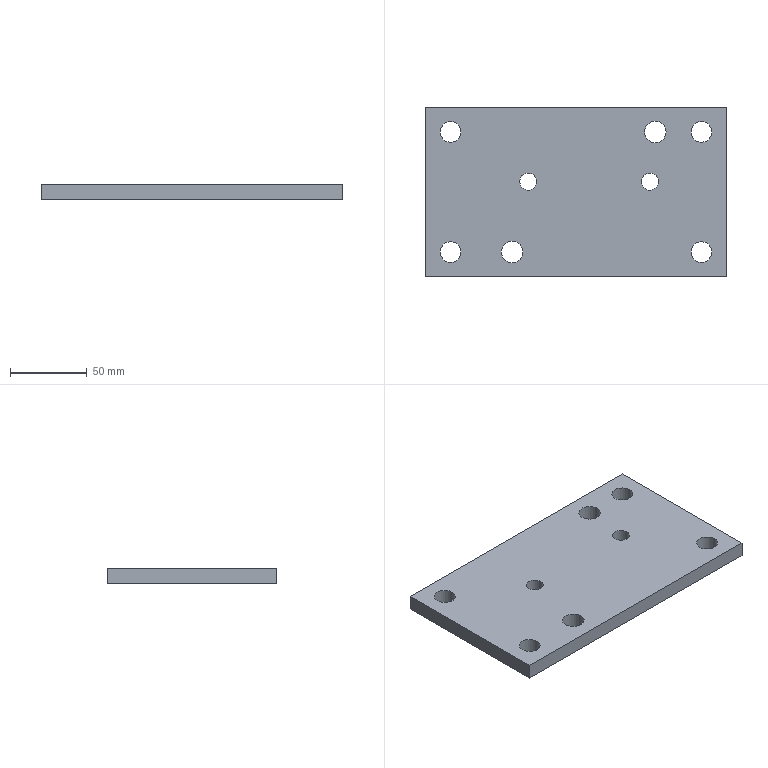Part | STEP file | lll_id2946_x_t | 1 solid | 14 faces | box 195 x 110 x 10 mm | volume 203787 mm3 | cylinder 8 | plane 6 | commonest cylinder face diameters 13.509 x4 11 x2 14 x2
STEP:
#1=CARTESIAN_POINT('',(1064.5,-23.25,102.5));
#2=VERTEX_POINT('',#1);
#3=CARTESIAN_POINT('',(1070.,-23.25,102.5));
#4=DIRECTION('',(0.,0.,-1.));
#5=DIRECTION('',(-1.,0.,0.));
#6=AXIS2_PLACEMENT_3D('',#3,#4,#5);
#7=CIRCLE('',#6,5.5);
#8=EDGE_CURVE('',#2,#2,#7,.T.);
#9=ORIENTED_EDGE('',*,*,#8,.F.);
#10=EDGE_LOOP('',(#9));
#11=FACE_BOUND('',#10,.T.);
#12=CARTESIAN_POINT('',(1064.5,-23.25,92.5));
#13=VERTEX_POINT('',#12);
#14=CARTESIAN_POINT('',(1070.,-23.25,92.5));
#15=DIRECTION('',(0.,0.,1.));
#16=DIRECTION('',(-1.,0.,0.));
#17=AXIS2_PLACEMENT_3D('',#14,#15,#16);
#18=CIRCLE('',#17,5.5);
#19=EDGE_CURVE('',#13,#13,#18,.T.);
#20=ORIENTED_EDGE('',*,*,#19,.F.);
#21=EDGE_LOOP('',(#20));
#22=FACE_BOUND('',#21,.T.);
#23=CARTESIAN_POINT('',(1070.,-23.25,217.5));
#24=DIRECTION('',(0.,0.,-1.));
#25=DIRECTION('',(-1.,0.,0.));
#26=AXIS2_PLACEMENT_3D('',#23,#24,#25);
#27=CYLINDRICAL_SURFACE('',#26,5.5);
#28=ADVANCED_FACE('',(#11,#22),#27,.F.);
#29=CARTESIAN_POINT('',(1145.5,9.,102.5));
#30=VERTEX_POINT('',#29);
#31=CARTESIAN_POINT('',(1152.5,9.,102.5));
#32=DIRECTION('',(0.,0.,-1.));
#33=DIRECTION('',(-1.,0.,0.));
#34=AXIS2_PLACEMENT_3D('',#31,#32,#33);
#35=CIRCLE('',#34,7.);
#36=EDGE_CURVE('',#30,#30,#35,.T.);
#37=ORIENTED_EDGE('',*,*,#36,.F.);
#38=EDGE_LOOP('',(#37));
#39=FACE_BOUND('',#38,.T.);
#40=CARTESIAN_POINT('',(1145.5,9.,92.5));
#41=VERTEX_POINT('',#40);
#42=CARTESIAN_POINT('',(1152.5,9.,92.5));
#43=DIRECTION('',(0.,0.,1.));
#44=DIRECTION('',(-1.,0.,0.));
#45=AXIS2_PLACEMENT_3D('',#42,#43,#44);
#46=CIRCLE('',#45,7.);
#47=EDGE_CURVE('',#41,#41,#46,.T.);
#48=ORIENTED_EDGE('',*,*,#47,.F.);
#49=EDGE_LOOP('',(#48));
#50=FACE_BOUND('',#49,.T.);
#51=CARTESIAN_POINT('',(1152.5,9.,92.5));
#52=DIRECTION('',(0.,0.,1.));
#53=DIRECTION('',(-1.,0.,0.));
#54=AXIS2_PLACEMENT_3D('',#51,#52,#53);
#55=CYLINDRICAL_SURFACE('',#54,7.);
#56=ADVANCED_FACE('',(#39,#50),#55,.F.);
#57=CARTESIAN_POINT('',(1012.745,9.,102.5));
#58=VERTEX_POINT('',#57);
#59=CARTESIAN_POINT('',(1019.5,9.,102.5));
#60=DIRECTION('',(0.,0.,1.));
#61=DIRECTION('',(-1.,0.,0.));
#62=AXIS2_PLACEMENT_3D('',#59,#60,#61);
#63=CIRCLE('',#62,6.755);
#64=EDGE_CURVE('',#58,#58,#63,.T.);
#65=ORIENTED_EDGE('',*,*,#64,.T.);
#66=EDGE_LOOP('',(#65));
#67=FACE_BOUND('',#66,.T.);
#68=CARTESIAN_POINT('',(1012.745,9.,92.5));
#69=VERTEX_POINT('',#68);
#70=CARTESIAN_POINT('',(1019.5,9.,92.5));
#71=DIRECTION('',(0.,0.,1.));
#72=DIRECTION('',(-1.,0.,0.));
#73=AXIS2_PLACEMENT_3D('',#70,#71,#72);
#74=CIRCLE('',#73,6.755);
#75=EDGE_CURVE('',#69,#69,#74,.T.);
#76=ORIENTED_EDGE('',*,*,#75,.F.);
#77=EDGE_LOOP('',(#76));
#78=FACE_BOUND('',#77,.T.);
#79=CARTESIAN_POINT('',(1019.5,9.,92.5));
#80=DIRECTION('',(0.,0.,1.));
#81=DIRECTION('',(-1.,0.,0.));
#82=AXIS2_PLACEMENT_3D('',#79,#80,#81);
#83=CYLINDRICAL_SURFACE('',#82,6.755);
#84=ADVANCED_FACE('',(#67,#78),#83,.F.);
#85=CARTESIAN_POINT('',(1175.745,9.,102.5));
#86=VERTEX_POINT('',#85);
#87=CARTESIAN_POINT('',(1182.5,9.,102.5));
#88=DIRECTION('',(0.,0.,1.));
#89=DIRECTION('',(-1.,0.,0.));
#90=AXIS2_PLACEMENT_3D('',#87,#88,#89);
#91=CIRCLE('',#90,6.755);
#92=EDGE_CURVE('',#86,#86,#91,.T.);
#93=ORIENTED_EDGE('',*,*,#92,.T.);
#94=EDGE_LOOP('',(#93));
#95=FACE_BOUND('',#94,.T.);
#96=CARTESIAN_POINT('',(1175.745,9.,92.5));
#97=VERTEX_POINT('',#96);
#98=CARTESIAN_POINT('',(1182.5,9.,92.5));
#99=DIRECTION('',(0.,0.,1.));
#100=DIRECTION('',(-1.,0.,0.));
#101=AXIS2_PLACEMENT_3D('',#98,#99,#100);
#102=CIRCLE('',#101,6.755);
#103=EDGE_CURVE('',#97,#97,#102,.T.);
#104=ORIENTED_EDGE('',*,*,#103,.F.);
#105=EDGE_LOOP('',(#104));
#106=FACE_BOUND('',#105,.T.);
#107=CARTESIAN_POINT('',(1182.5,9.,92.5));
#108=DIRECTION('',(0.,0.,1.));
#109=DIRECTION('',(-1.,0.,0.));
#110=AXIS2_PLACEMENT_3D('',#107,#108,#109);
#111=CYLINDRICAL_SURFACE('',#110,6.755);
#112=ADVANCED_FACE('',(#95,#106),#111,.F.);
#113=CARTESIAN_POINT('',(1003.5,25.,102.5));
#114=VERTEX_POINT('',#113);
#115=CARTESIAN_POINT('',(1003.5,-85.,102.5));
#116=VERTEX_POINT('',#115);
#117=CARTESIAN_POINT('',(1003.5,-30.,102.5));
#118=DIRECTION('',(0.,-1.,0.));
#119=VECTOR('',#118,1.);
#120=LINE('',#117,#119);
#121=EDGE_CURVE('',#114,#116,#120,.T.);
#122=ORIENTED_EDGE('',*,*,#121,.F.);
#123=CARTESIAN_POINT('',(1003.5,25.,92.5));
#124=VERTEX_POINT('',#123);
#125=CARTESIAN_POINT('',(1003.5,25.,92.5));
#126=DIRECTION('',(0.,0.,1.));
#127=VECTOR('',#126,1.);
#128=LINE('',#125,#127);
#129=EDGE_CURVE('',#124,#114,#128,.T.);
#130=ORIENTED_EDGE('',*,*,#129,.F.);
#131=CARTESIAN_POINT('',(1003.5,-85.,92.5));
#132=VERTEX_POINT('',#131);
#133=CARTESIAN_POINT('',(1003.5,-30.,92.5));
#134=DIRECTION('',(0.,-1.,0.));
#135=VECTOR('',#134,1.);
#136=LINE('',#133,#135);
#137=EDGE_CURVE('',#124,#132,#136,.T.);
#138=ORIENTED_EDGE('',*,*,#137,.T.);
#139=CARTESIAN_POINT('',(1003.5,-85.,92.5));
#140=DIRECTION('',(0.,0.,1.));
#141=VECTOR('',#140,1.);
#142=LINE('',#139,#141);
#143=EDGE_CURVE('',#132,#116,#142,.T.);
#144=ORIENTED_EDGE('',*,*,#143,.T.);
#145=EDGE_LOOP('',(#122,#130,#138,#144));
#146=FACE_OUTER_BOUND('',#145,.T.);
#147=CARTESIAN_POINT('',(1003.5,-30.,92.5));
#148=DIRECTION('',(-1.,0.,0.));
#149=DIRECTION('',(0.,0.,-1.));
#150=AXIS2_PLACEMENT_3D('',#147,#148,#149);
#151=PLANE('',#150);
#152=ADVANCED_FACE('',(#146),#151,.T.);
#153=CARTESIAN_POINT('',(1198.5,-85.,102.5));
#154=VERTEX_POINT('',#153);
#155=CARTESIAN_POINT('',(1101.,-85.,102.5));
#156=DIRECTION('',(-1.,0.,0.));
#157=VECTOR('',#156,1.);
#158=LINE('',#155,#157);
#159=EDGE_CURVE('',#154,#116,#158,.T.);
#160=ORIENTED_EDGE('',*,*,#159,.T.);
#161=ORIENTED_EDGE('',*,*,#143,.F.);
#162=CARTESIAN_POINT('',(1198.5,-85.,92.5));
#163=VERTEX_POINT('',#162);
#164=CARTESIAN_POINT('',(1101.,-85.,92.5));
#165=DIRECTION('',(1.,0.,0.));
#166=VECTOR('',#165,1.);
#167=LINE('',#164,#166);
#168=EDGE_CURVE('',#132,#163,#167,.T.);
#169=ORIENTED_EDGE('',*,*,#168,.T.);
#170=CARTESIAN_POINT('',(1198.5,-85.,92.5));
#171=DIRECTION('',(0.,0.,1.));
#172=VECTOR('',#171,1.);
#173=LINE('',#170,#172);
#174=EDGE_CURVE('',#163,#154,#173,.T.);
#175=ORIENTED_EDGE('',*,*,#174,.T.);
#176=EDGE_LOOP('',(#160,#161,#169,#175));
#177=FACE_OUTER_BOUND('',#176,.T.);
#178=CARTESIAN_POINT('',(1101.,-85.,92.5));
#179=DIRECTION('',(0.,-1.,0.));
#180=DIRECTION('',(0.,0.,1.));
#181=AXIS2_PLACEMENT_3D('',#178,#179,#180);
#182=PLANE('',#181);
#183=ADVANCED_FACE('',(#177),#182,.T.);
#184=CARTESIAN_POINT('',(1198.5,25.,102.5));
#185=VERTEX_POINT('',#184);
#186=CARTESIAN_POINT('',(1198.5,-30.,102.5));
#187=DIRECTION('',(0.,1.,0.));
#188=VECTOR('',#187,1.);
#189=LINE('',#186,#188);
#190=EDGE_CURVE('',#154,#185,#189,.T.);
#191=ORIENTED_EDGE('',*,*,#190,.F.);
#192=ORIENTED_EDGE('',*,*,#174,.F.);
#193=CARTESIAN_POINT('',(1198.5,25.,92.5));
#194=VERTEX_POINT('',#193);
#195=CARTESIAN_POINT('',(1198.5,-30.,92.5));
#196=DIRECTION('',(0.,1.,0.));
#197=VECTOR('',#196,1.);
#198=LINE('',#195,#197);
#199=EDGE_CURVE('',#163,#194,#198,.T.);
#200=ORIENTED_EDGE('',*,*,#199,.T.);
#201=CARTESIAN_POINT('',(1198.5,25.,92.5));
#202=DIRECTION('',(0.,0.,1.));
#203=VECTOR('',#202,1.);
#204=LINE('',#201,#203);
#205=EDGE_CURVE('',#194,#185,#204,.T.);
#206=ORIENTED_EDGE('',*,*,#205,.T.);
#207=EDGE_LOOP('',(#191,#192,#200,#206));
#208=FACE_OUTER_BOUND('',#207,.T.);
#209=CARTESIAN_POINT('',(1198.5,-30.,92.5));
#210=DIRECTION('',(1.,0.,0.));
#211=DIRECTION('',(0.,0.,1.));
#212=AXIS2_PLACEMENT_3D('',#209,#210,#211);
#213=PLANE('',#212);
#214=ADVANCED_FACE('',(#208),#213,.T.);
#215=CARTESIAN_POINT('',(1101.,25.,102.5));
#216=DIRECTION('',(-1.,0.,0.));
#217=VECTOR('',#216,1.);
#218=LINE('',#215,#217);
#219=EDGE_CURVE('',#185,#114,#218,.T.);
#220=ORIENTED_EDGE('',*,*,#219,.F.);
#221=ORIENTED_EDGE('',*,*,#205,.F.);
#222=CARTESIAN_POINT('',(1101.,25.,92.5));
#223=DIRECTION('',(-1.,0.,0.));
#224=VECTOR('',#223,1.);
#225=LINE('',#222,#224);
#226=EDGE_CURVE('',#194,#124,#225,.T.);
#227=ORIENTED_EDGE('',*,*,#226,.T.);
#228=ORIENTED_EDGE('',*,*,#129,.T.);
#229=EDGE_LOOP('',(#220,#221,#227,#228));
#230=FACE_OUTER_BOUND('',#229,.T.);
#231=CARTESIAN_POINT('',(1101.,25.,92.5));
#232=DIRECTION('',(0.,1.,0.));
#233=DIRECTION('',(0.,0.,-1.));
#234=AXIS2_PLACEMENT_3D('',#231,#232,#233);
#235=PLANE('',#234);
#236=ADVANCED_FACE('',(#230),#235,.T.);
#237=CARTESIAN_POINT('',(1012.745,-69.,102.5));
#238=VERTEX_POINT('',#237);
#239=CARTESIAN_POINT('',(1019.5,-69.,102.5));
#240=DIRECTION('',(0.,0.,-1.));
#241=DIRECTION('',(-1.,0.,0.));
#242=AXIS2_PLACEMENT_3D('',#239,#240,#241);
#243=CIRCLE('',#242,6.755);
#244=EDGE_CURVE('',#238,#238,#243,.T.);
#245=ORIENTED_EDGE('',*,*,#244,.F.);
#246=EDGE_LOOP('',(#245));
#247=FACE_BOUND('',#246,.T.);
#248=CARTESIAN_POINT('',(1012.745,-69.,92.5));
#249=VERTEX_POINT('',#248);
#250=CARTESIAN_POINT('',(1019.5,-69.,92.5));
#251=DIRECTION('',(0.,0.,1.));
#252=DIRECTION('',(-1.,0.,0.));
#253=AXIS2_PLACEMENT_3D('',#250,#251,#252);
#254=CIRCLE('',#253,6.755);
#255=EDGE_CURVE('',#249,#249,#254,.T.);
#256=ORIENTED_EDGE('',*,*,#255,.F.);
#257=EDGE_LOOP('',(#256));
#258=FACE_BOUND('',#257,.T.);
#259=CARTESIAN_POINT('',(1019.5,-69.,92.5));
#260=DIRECTION('',(0.,0.,1.));
#261=DIRECTION('',(-1.,0.,0.));
#262=AXIS2_PLACEMENT_3D('',#259,#260,#261);
#263=CYLINDRICAL_SURFACE('',#262,6.755);
#264=ADVANCED_FACE('',(#247,#258),#263,.F.);
#265=CARTESIAN_POINT('',(1175.745,-69.,102.5));
#266=VERTEX_POINT('',#265);
#267=CARTESIAN_POINT('',(1182.5,-69.,102.5));
#268=DIRECTION('',(0.,0.,1.));
#269=DIRECTION('',(-1.,0.,0.));
#270=AXIS2_PLACEMENT_3D('',#267,#268,#269);
#271=CIRCLE('',#270,6.755);
#272=EDGE_CURVE('',#266,#266,#271,.T.);
#273=ORIENTED_EDGE('',*,*,#272,.T.);
#274=EDGE_LOOP('',(#273));
#275=FACE_BOUND('',#274,.T.);
#276=CARTESIAN_POINT('',(1175.745,-69.,92.5));
#277=VERTEX_POINT('',#276);
#278=CARTESIAN_POINT('',(1182.5,-69.,92.5));
#279=DIRECTION('',(0.,0.,1.));
#280=DIRECTION('',(-1.,0.,0.));
#281=AXIS2_PLACEMENT_3D('',#278,#279,#280);
#282=CIRCLE('',#281,6.755);
#283=EDGE_CURVE('',#277,#277,#282,.T.);
#284=ORIENTED_EDGE('',*,*,#283,.F.);
#285=EDGE_LOOP('',(#284));
#286=FACE_BOUND('',#285,.T.);
#287=CARTESIAN_POINT('',(1182.5,-69.,92.5));
#288=DIRECTION('',(0.,0.,1.));
#289=DIRECTION('',(-1.,0.,0.));
#290=AXIS2_PLACEMENT_3D('',#287,#288,#289);
#291=CYLINDRICAL_SURFACE('',#290,6.755);
#292=ADVANCED_FACE('',(#275,#286),#291,.F.);
#293=CARTESIAN_POINT('',(1052.5,-69.,102.5));
#294=VERTEX_POINT('',#293);
#295=CARTESIAN_POINT('',(1059.5,-69.,102.5));
#296=DIRECTION('',(0.,0.,1.));
#297=DIRECTION('',(-1.,0.,0.));
#298=AXIS2_PLACEMENT_3D('',#295,#296,#297);
#299=CIRCLE('',#298,7.);
#300=EDGE_CURVE('',#294,#294,#299,.T.);
#301=ORIENTED_EDGE('',*,*,#300,.T.);
#302=EDGE_LOOP('',(#301));
#303=FACE_BOUND('',#302,.T.);
#304=CARTESIAN_POINT('',(1052.5,-69.,92.5));
#305=VERTEX_POINT('',#304);
#306=CARTESIAN_POINT('',(1059.5,-69.,92.5));
#307=DIRECTION('',(0.,0.,1.));
#308=DIRECTION('',(-1.,0.,0.));
#309=AXIS2_PLACEMENT_3D('',#306,#307,#308);
#310=CIRCLE('',#309,7.);
#311=EDGE_CURVE('',#305,#305,#310,.T.);
#312=ORIENTED_EDGE('',*,*,#311,.F.);
#313=EDGE_LOOP('',(#312));
#314=FACE_BOUND('',#313,.T.);
#315=CARTESIAN_POINT('',(1059.5,-69.,92.5));
#316=DIRECTION('',(0.,0.,1.));
#317=DIRECTION('',(-1.,0.,0.));
#318=AXIS2_PLACEMENT_3D('',#315,#316,#317);
#319=CYLINDRICAL_SURFACE('',#318,7.);
#320=ADVANCED_FACE('',(#303,#314),#319,.F.);
#321=CARTESIAN_POINT('',(1143.5,-23.25,92.5));
#322=VERTEX_POINT('',#321);
#323=CARTESIAN_POINT('',(1149.,-23.25,92.5));
#324=DIRECTION('',(0.,0.,-1.));
#325=DIRECTION('',(-1.,0.,0.));
#326=AXIS2_PLACEMENT_3D('',#323,#324,#325);
#327=CIRCLE('',#326,5.5);
#328=EDGE_CURVE('',#322,#322,#327,.T.);
#329=ORIENTED_EDGE('',*,*,#328,.F.);
#330=EDGE_LOOP('',(#329));
#331=FACE_BOUND('',#330,.T.);
#332=ORIENTED_EDGE('',*,*,#311,.T.);
#333=EDGE_LOOP('',(#332));
#334=FACE_BOUND('',#333,.T.);
#335=ORIENTED_EDGE('',*,*,#283,.T.);
#336=EDGE_LOOP('',(#335));
#337=FACE_BOUND('',#336,.T.);
#338=ORIENTED_EDGE('',*,*,#255,.T.);
#339=EDGE_LOOP('',(#338));
#340=FACE_BOUND('',#339,.T.);
#341=ORIENTED_EDGE('',*,*,#137,.F.);
#342=ORIENTED_EDGE('',*,*,#226,.F.);
#343=ORIENTED_EDGE('',*,*,#199,.F.);
#344=ORIENTED_EDGE('',*,*,#168,.F.);
#345=EDGE_LOOP('',(#341,#342,#343,#344));
#346=FACE_BOUND('',#345,.T.);
#347=ORIENTED_EDGE('',*,*,#103,.T.);
#348=EDGE_LOOP('',(#347));
#349=FACE_BOUND('',#348,.T.);
#350=ORIENTED_EDGE('',*,*,#75,.T.);
#351=EDGE_LOOP('',(#350));
#352=FACE_BOUND('',#351,.T.);
#353=ORIENTED_EDGE('',*,*,#47,.T.);
#354=EDGE_LOOP('',(#353));
#355=FACE_BOUND('',#354,.T.);
#356=ORIENTED_EDGE('',*,*,#19,.T.);
#357=EDGE_LOOP('',(#356));
#358=FACE_BOUND('',#357,.T.);
#359=CARTESIAN_POINT('',(1101.,-30.,92.5));
#360=DIRECTION('',(0.,0.,-1.));
#361=DIRECTION('',(1.,0.,0.));
#362=AXIS2_PLACEMENT_3D('',#359,#360,#361);
#363=PLANE('',#362);
#364=ADVANCED_FACE('',(#331,#334,#337,#340,#346,#349,#352,#355,#358),#363,.T.);
#365=CARTESIAN_POINT('',(1143.5,-23.25,102.5));
#366=VERTEX_POINT('',#365);
#367=CARTESIAN_POINT('',(1149.,-23.25,102.5));
#368=DIRECTION('',(0.,0.,-1.));
#369=DIRECTION('',(-1.,0.,0.));
#370=AXIS2_PLACEMENT_3D('',#367,#368,#369);
#371=CIRCLE('',#370,5.5);
#372=EDGE_CURVE('',#366,#366,#371,.T.);
#373=ORIENTED_EDGE('',*,*,#372,.F.);
#374=EDGE_LOOP('',(#373));
#375=FACE_BOUND('',#374,.T.);
#376=ORIENTED_EDGE('',*,*,#328,.T.);
#377=EDGE_LOOP('',(#376));
#378=FACE_BOUND('',#377,.T.);
#379=CARTESIAN_POINT('',(1149.,-23.25,217.5));
#380=DIRECTION('',(0.,0.,-1.));
#381=DIRECTION('',(-1.,0.,0.));
#382=AXIS2_PLACEMENT_3D('',#379,#380,#381);
#383=CYLINDRICAL_SURFACE('',#382,5.5);
#384=ADVANCED_FACE('',(#375,#378),#383,.F.);
#385=ORIENTED_EDGE('',*,*,#219,.T.);
#386=ORIENTED_EDGE('',*,*,#121,.T.);
#387=ORIENTED_EDGE('',*,*,#159,.F.);
#388=ORIENTED_EDGE('',*,*,#190,.T.);
#389=EDGE_LOOP('',(#385,#386,#387,#388));
#390=FACE_BOUND('',#389,.T.);
#391=ORIENTED_EDGE('',*,*,#244,.T.);
#392=EDGE_LOOP('',(#391));
#393=FACE_BOUND('',#392,.T.);
#394=ORIENTED_EDGE('',*,*,#272,.F.);
#395=EDGE_LOOP('',(#394));
#396=FACE_BOUND('',#395,.T.);
#397=ORIENTED_EDGE('',*,*,#300,.F.);
#398=EDGE_LOOP('',(#397));
#399=FACE_BOUND('',#398,.T.);
#400=ORIENTED_EDGE('',*,*,#8,.T.);
#401=EDGE_LOOP('',(#400));
#402=FACE_BOUND('',#401,.T.);
#403=ORIENTED_EDGE('',*,*,#372,.T.);
#404=EDGE_LOOP('',(#403));
#405=FACE_BOUND('',#404,.T.);
#406=ORIENTED_EDGE('',*,*,#36,.T.);
#407=EDGE_LOOP('',(#406));
#408=FACE_BOUND('',#407,.T.);
#409=ORIENTED_EDGE('',*,*,#64,.F.);
#410=EDGE_LOOP('',(#409));
#411=FACE_BOUND('',#410,.T.);
#412=ORIENTED_EDGE('',*,*,#92,.F.);
#413=EDGE_LOOP('',(#412));
#414=FACE_BOUND('',#413,.T.);
#415=CARTESIAN_POINT('',(741.5,-0.002299,102.5));
#416=DIRECTION('',(0.,0.,-1.));
#417=DIRECTION('',(-1.,0.,0.));
#418=AXIS2_PLACEMENT_3D('',#415,#416,#417);
#419=PLANE('',#418);
#420=ADVANCED_FACE('',(#390,#393,#396,#399,#402,#405,#408,#411,#414),#419,.F.);
#421=CLOSED_SHELL('',(#28,#56,#84,#112,#152,#183,#214,#236,#264,#292,#320,#364,#384,#420));
#422=MANIFOLD_SOLID_BREP('',#421);
#423=(LENGTH_UNIT()NAMED_UNIT(*)SI_UNIT(.MILLI.,.METRE.));
#424=UNCERTAINTY_MEASURE_WITH_UNIT(LENGTH_MEASURE(0.00002),#423,'','');
#425=(NAMED_UNIT(*)PLANE_ANGLE_UNIT()SI_UNIT($,.RADIAN.));
#426=PLANE_ANGLE_MEASURE_WITH_UNIT(PLANE_ANGLE_MEASURE(0.01745),#425);
#427=DIMENSIONAL_EXPONENTS(0.,0.,0.,0.,0.,0.,0.);
#428=(CONVERSION_BASED_UNIT('DEGREE',#426)NAMED_UNIT(#427)PLANE_ANGLE_UNIT());
#429=(NAMED_UNIT(*)SI_UNIT($,.STERADIAN.)SOLID_ANGLE_UNIT());
#430=(GEOMETRIC_REPRESENTATION_CONTEXT(3)GLOBAL_UNCERTAINTY_ASSIGNED_CONTEXT((#424))GLOBAL_UNIT_ASSIGNED_CONTEXT((#423,#428,#429))REPRESENTATION_CONTEXT('',''));
#431=ADVANCED_BREP_SHAPE_REPRESENTATION('',(#422),#430);